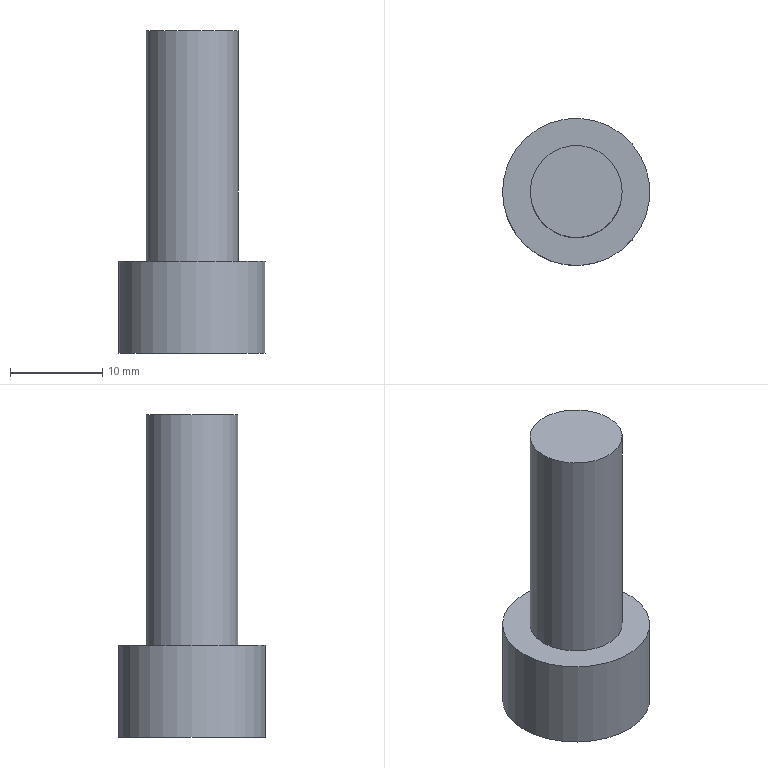Part | STEP file | 1 solid | 12 faces | box 16 x 16 x 35 mm | volume 3608 mm3 | plane 10 | cylinder 2 | commonest cylinder face diameters 10 x1 16 x1
STEP:
#1=CARTESIAN_POINT('',(0.,0.,0.));
#2=DIRECTION('',(0.,0.,1.));
#3=DIRECTION('',(1.,0.,0.));
#4=AXIS2_PLACEMENT_3D('',#1,#2,#3);
#5=CARTESIAN_POINT('',(1674.247,277.48,-164.381));
#6=VERTEX_POINT('',#5);
#7=CARTESIAN_POINT('',(1682.247,277.48,-164.381));
#8=DIRECTION('',(0.,0.,-1.));
#9=DIRECTION('',(-1.,0.,0.));
#10=AXIS2_PLACEMENT_3D('',#7,#8,#9);
#11=CIRCLE('',#10,8.);
#12=CARTESIAN_POINT('',(1674.247,277.48,-164.381));
#13=DIRECTION('',(0.,0.,1.));
#14=DIRECTION('',(1.,0.,0.));
#15=AXIS2_PLACEMENT_3D('',#12,#13,#14);
#16=PLANE('',#15);
#17=CARTESIAN_POINT('',(0.,0.));
#18=CARTESIAN_POINT('',(0.,13.856));
#19=CARTESIAN_POINT('',(12.,6.928));
#20=CARTESIAN_POINT('',(24.,0.));
#21=CARTESIAN_POINT('',(12.,-6.928));
#22=CARTESIAN_POINT('',(0.,-13.856));
#23=CARTESIAN_POINT('',(0.,0.));
#24=(BOUNDED_CURVE()B_SPLINE_CURVE(2,(#17,#18,#19,#20,#21,#22,#23),.UNSPECIFIED.,.T.,.F.)B_SPLINE_CURVE_WITH_KNOTS((1,2,2,2,2,1),(-2.094,0.,2.094,4.189,6.283,8.378),.UNSPECIFIED.)CURVE()GEOMETRIC_REPRESENTATION_ITEM()RATIONAL_B_SPLINE_CURVE((1.,0.5,1.,0.5,1.,0.5,1.))REPRESENTATION_ITEM(''));
#25=(GEOMETRIC_REPRESENTATION_CONTEXT(2)PARAMETRIC_REPRESENTATION_CONTEXT()REPRESENTATION_CONTEXT('',''));
#26=DEFINITIONAL_REPRESENTATION('',(#24),#25);
#27=PCURVE('',#16,#26);
#28=CARTESIAN_POINT('',(1682.247,277.48,-145.481));
#29=DIRECTION('',(0.,0.,-1.));
#30=DIRECTION('',(-1.,0.,0.));
#31=AXIS2_PLACEMENT_3D('',#28,#29,#30);
#32=CYLINDRICAL_SURFACE('',#31,8.);
#33=CARTESIAN_POINT('',(0.,18.9));
#34=DIRECTION('',(1.,0.));
#35=VECTOR('',#34,1.);
#36=LINE('',#33,#35);
#37=(GEOMETRIC_REPRESENTATION_CONTEXT(2)PARAMETRIC_REPRESENTATION_CONTEXT()REPRESENTATION_CONTEXT('',''));
#38=DEFINITIONAL_REPRESENTATION('',(#36),#37);
#39=PCURVE('',#32,#38);
#40=SURFACE_CURVE('',#11,(#27,#39),.PCURVE_S1.);
#41=EDGE_CURVE('',#6,#6,#40,.T.);
#42=ORIENTED_EDGE('',*,*,#41,.T.);
#43=EDGE_LOOP('',(#42));
#44=FACE_BOUND('',#43,.T.);
#45=CARTESIAN_POINT('',(1684.557,281.48,-164.381));
#46=VERTEX_POINT('',#45);
#47=CARTESIAN_POINT('',(1679.938,281.48,-164.381));
#48=VERTEX_POINT('',#47);
#49=CARTESIAN_POINT('',(1684.557,281.48,-164.381));
#50=DIRECTION('',(-1.,0.,0.));
#51=VECTOR('',#50,1.);
#52=LINE('',#49,#51);
#53=CARTESIAN_POINT('',(10.309,4.));
#54=DIRECTION('',(-1.,0.));
#55=VECTOR('',#54,1.);
#56=LINE('',#53,#55);
#57=(GEOMETRIC_REPRESENTATION_CONTEXT(2)PARAMETRIC_REPRESENTATION_CONTEXT()REPRESENTATION_CONTEXT('',''));
#58=DEFINITIONAL_REPRESENTATION('',(#56),#57);
#59=PCURVE('',#16,#58);
#60=CARTESIAN_POINT('',(1684.557,281.48,-157.781));
#61=DIRECTION('',(0.,-1.,0.));
#62=DIRECTION('',(-1.,0.,0.));
#63=AXIS2_PLACEMENT_3D('',#60,#61,#62);
#64=PLANE('',#63);
#65=CARTESIAN_POINT('',(0.,6.6));
#66=DIRECTION('',(1.,0.));
#67=VECTOR('',#66,1.);
#68=LINE('',#65,#67);
#69=(GEOMETRIC_REPRESENTATION_CONTEXT(2)PARAMETRIC_REPRESENTATION_CONTEXT()REPRESENTATION_CONTEXT('',''));
#70=DEFINITIONAL_REPRESENTATION('',(#68),#69);
#71=PCURVE('',#64,#70);
#72=SURFACE_CURVE('',#52,(#59,#71),.PCURVE_S1.);
#73=EDGE_CURVE('',#46,#48,#72,.T.);
#74=ORIENTED_EDGE('',*,*,#73,.T.);
#75=CARTESIAN_POINT('',(1677.628,277.48,-164.381));
#76=VERTEX_POINT('',#75);
#77=CARTESIAN_POINT('',(1679.938,281.48,-164.381));
#78=DIRECTION('',(-0.5,-0.866,0.));
#79=VECTOR('',#78,1.);
#80=LINE('',#77,#79);
#81=CARTESIAN_POINT('',(5.691,4.));
#82=DIRECTION('',(-0.5,-0.866));
#83=VECTOR('',#82,1.);
#84=LINE('',#81,#83);
#85=(GEOMETRIC_REPRESENTATION_CONTEXT(2)PARAMETRIC_REPRESENTATION_CONTEXT()REPRESENTATION_CONTEXT('',''));
#86=DEFINITIONAL_REPRESENTATION('',(#84),#85);
#87=PCURVE('',#16,#86);
#88=CARTESIAN_POINT('',(1679.938,281.48,-157.781));
#89=DIRECTION('',(0.866,-0.5,0.));
#90=DIRECTION('',(-0.5,-0.866,0.));
#91=AXIS2_PLACEMENT_3D('',#88,#89,#90);
#92=PLANE('',#91);
#93=CARTESIAN_POINT('',(0.,6.6));
#94=DIRECTION('',(1.,0.));
#95=VECTOR('',#94,1.);
#96=LINE('',#93,#95);
#97=(GEOMETRIC_REPRESENTATION_CONTEXT(2)PARAMETRIC_REPRESENTATION_CONTEXT()REPRESENTATION_CONTEXT('',''));
#98=DEFINITIONAL_REPRESENTATION('',(#96),#97);
#99=PCURVE('',#92,#98);
#100=SURFACE_CURVE('',#80,(#87,#99),.PCURVE_S1.);
#101=EDGE_CURVE('',#48,#76,#100,.T.);
#102=ORIENTED_EDGE('',*,*,#101,.T.);
#103=CARTESIAN_POINT('',(1679.938,273.48,-164.381));
#104=VERTEX_POINT('',#103);
#105=CARTESIAN_POINT('',(1677.628,277.48,-164.381));
#106=DIRECTION('',(0.5,-0.866,0.));
#107=VECTOR('',#106,1.);
#108=LINE('',#105,#107);
#109=CARTESIAN_POINT('',(3.381,0.));
#110=DIRECTION('',(0.5,-0.866));
#111=VECTOR('',#110,1.);
#112=LINE('',#109,#111);
#113=(GEOMETRIC_REPRESENTATION_CONTEXT(2)PARAMETRIC_REPRESENTATION_CONTEXT()REPRESENTATION_CONTEXT('',''));
#114=DEFINITIONAL_REPRESENTATION('',(#112),#113);
#115=PCURVE('',#16,#114);
#116=CARTESIAN_POINT('',(1677.628,277.48,-157.781));
#117=DIRECTION('',(0.866,0.5,0.));
#118=DIRECTION('',(0.5,-0.866,0.));
#119=AXIS2_PLACEMENT_3D('',#116,#117,#118);
#120=PLANE('',#119);
#121=CARTESIAN_POINT('',(0.,6.6));
#122=DIRECTION('',(1.,0.));
#123=VECTOR('',#122,1.);
#124=LINE('',#121,#123);
#125=(GEOMETRIC_REPRESENTATION_CONTEXT(2)PARAMETRIC_REPRESENTATION_CONTEXT()REPRESENTATION_CONTEXT('',''));
#126=DEFINITIONAL_REPRESENTATION('',(#124),#125);
#127=PCURVE('',#120,#126);
#128=SURFACE_CURVE('',#108,(#115,#127),.PCURVE_S1.);
#129=EDGE_CURVE('',#76,#104,#128,.T.);
#130=ORIENTED_EDGE('',*,*,#129,.T.);
#131=CARTESIAN_POINT('',(1684.557,273.48,-164.381));
#132=VERTEX_POINT('',#131);
#133=CARTESIAN_POINT('',(1679.938,273.48,-164.381));
#134=DIRECTION('',(1.,0.,0.));
#135=VECTOR('',#134,1.);
#136=LINE('',#133,#135);
#137=CARTESIAN_POINT('',(5.691,-4.));
#138=DIRECTION('',(1.,0.));
#139=VECTOR('',#138,1.);
#140=LINE('',#137,#139);
#141=(GEOMETRIC_REPRESENTATION_CONTEXT(2)PARAMETRIC_REPRESENTATION_CONTEXT()REPRESENTATION_CONTEXT('',''));
#142=DEFINITIONAL_REPRESENTATION('',(#140),#141);
#143=PCURVE('',#16,#142);
#144=CARTESIAN_POINT('',(1679.938,273.48,-157.781));
#145=DIRECTION('',(0.,1.,0.));
#146=DIRECTION('',(1.,0.,0.));
#147=AXIS2_PLACEMENT_3D('',#144,#145,#146);
#148=PLANE('',#147);
#149=CARTESIAN_POINT('',(0.,6.6));
#150=DIRECTION('',(1.,0.));
#151=VECTOR('',#150,1.);
#152=LINE('',#149,#151);
#153=(GEOMETRIC_REPRESENTATION_CONTEXT(2)PARAMETRIC_REPRESENTATION_CONTEXT()REPRESENTATION_CONTEXT('',''));
#154=DEFINITIONAL_REPRESENTATION('',(#152),#153);
#155=PCURVE('',#148,#154);
#156=SURFACE_CURVE('',#136,(#143,#155),.PCURVE_S1.);
#157=EDGE_CURVE('',#104,#132,#156,.T.);
#158=ORIENTED_EDGE('',*,*,#157,.T.);
#159=CARTESIAN_POINT('',(1686.866,277.48,-164.381));
#160=VERTEX_POINT('',#159);
#161=CARTESIAN_POINT('',(1684.557,273.48,-164.381));
#162=DIRECTION('',(0.5,0.866,0.));
#163=VECTOR('',#162,1.);
#164=LINE('',#161,#163);
#165=CARTESIAN_POINT('',(10.309,-4.));
#166=DIRECTION('',(0.5,0.866));
#167=VECTOR('',#166,1.);
#168=LINE('',#165,#167);
#169=(GEOMETRIC_REPRESENTATION_CONTEXT(2)PARAMETRIC_REPRESENTATION_CONTEXT()REPRESENTATION_CONTEXT('',''));
#170=DEFINITIONAL_REPRESENTATION('',(#168),#169);
#171=PCURVE('',#16,#170);
#172=CARTESIAN_POINT('',(1684.557,273.48,-157.781));
#173=DIRECTION('',(-0.866,0.5,0.));
#174=DIRECTION('',(0.5,0.866,0.));
#175=AXIS2_PLACEMENT_3D('',#172,#173,#174);
#176=PLANE('',#175);
#177=CARTESIAN_POINT('',(0.,6.6));
#178=DIRECTION('',(1.,0.));
#179=VECTOR('',#178,1.);
#180=LINE('',#177,#179);
#181=(GEOMETRIC_REPRESENTATION_CONTEXT(2)PARAMETRIC_REPRESENTATION_CONTEXT()REPRESENTATION_CONTEXT('',''));
#182=DEFINITIONAL_REPRESENTATION('',(#180),#181);
#183=PCURVE('',#176,#182);
#184=SURFACE_CURVE('',#164,(#171,#183),.PCURVE_S1.);
#185=EDGE_CURVE('',#132,#160,#184,.T.);
#186=ORIENTED_EDGE('',*,*,#185,.T.);
#187=CARTESIAN_POINT('',(1686.866,277.48,-164.381));
#188=DIRECTION('',(-0.5,0.866,0.));
#189=VECTOR('',#188,1.);
#190=LINE('',#187,#189);
#191=CARTESIAN_POINT('',(12.619,0.));
#192=DIRECTION('',(-0.5,0.866));
#193=VECTOR('',#192,1.);
#194=LINE('',#191,#193);
#195=(GEOMETRIC_REPRESENTATION_CONTEXT(2)PARAMETRIC_REPRESENTATION_CONTEXT()REPRESENTATION_CONTEXT('',''));
#196=DEFINITIONAL_REPRESENTATION('',(#194),#195);
#197=PCURVE('',#16,#196);
#198=CARTESIAN_POINT('',(1686.866,277.48,-157.781));
#199=DIRECTION('',(-0.866,-0.5,0.));
#200=DIRECTION('',(-0.5,0.866,0.));
#201=AXIS2_PLACEMENT_3D('',#198,#199,#200);
#202=PLANE('',#201);
#203=CARTESIAN_POINT('',(0.,6.6));
#204=DIRECTION('',(1.,0.));
#205=VECTOR('',#204,1.);
#206=LINE('',#203,#205);
#207=(GEOMETRIC_REPRESENTATION_CONTEXT(2)PARAMETRIC_REPRESENTATION_CONTEXT()REPRESENTATION_CONTEXT('',''));
#208=DEFINITIONAL_REPRESENTATION('',(#206),#207);
#209=PCURVE('',#202,#208);
#210=SURFACE_CURVE('',#190,(#197,#209),.PCURVE_S1.);
#211=EDGE_CURVE('',#160,#46,#210,.T.);
#212=ORIENTED_EDGE('',*,*,#211,.T.);
#213=EDGE_LOOP('',(#74,#102,#130,#158,#186,#212));
#214=FACE_BOUND('',#213,.T.);
#215=ADVANCED_FACE('',(#44,#214),#16,.F.);
#216=ORIENTED_EDGE('',*,*,#41,.F.);
#217=CARTESIAN_POINT('',(1674.247,277.48,-154.381));
#218=VERTEX_POINT('',#217);
#219=CARTESIAN_POINT('',(1674.247,277.48,-154.381));
#220=CARTESIAN_POINT('',(1674.247,277.48,-164.381));
#221=B_SPLINE_CURVE_WITH_KNOTS('',1,(#219,#220),.UNSPECIFIED.,.F.,.F.,(2,2),(8.9,18.9),.PIECEWISE_BEZIER_KNOTS.);
#222=CARTESIAN_POINT('',(0.,0.));
#223=DIRECTION('',(0.,1.));
#224=VECTOR('',#223,1.);
#225=LINE('',#222,#224);
#226=(GEOMETRIC_REPRESENTATION_CONTEXT(2)PARAMETRIC_REPRESENTATION_CONTEXT()REPRESENTATION_CONTEXT('',''));
#227=DEFINITIONAL_REPRESENTATION('',(#225),#226);
#228=PCURVE('',#32,#227);
#229=CARTESIAN_POINT('',(6.283,0.));
#230=DIRECTION('',(0.,1.));
#231=VECTOR('',#230,1.);
#232=LINE('',#229,#231);
#233=(GEOMETRIC_REPRESENTATION_CONTEXT(2)PARAMETRIC_REPRESENTATION_CONTEXT()REPRESENTATION_CONTEXT('',''));
#234=DEFINITIONAL_REPRESENTATION('',(#232),#233);
#235=PCURVE('',#32,#234);
#236=SEAM_CURVE('',#221,(#228,#235),.PCURVE_S1.);
#237=EDGE_CURVE('',#218,#6,#236,.T.);
#238=ORIENTED_EDGE('',*,*,#237,.F.);
#239=CARTESIAN_POINT('',(1682.247,277.48,-154.381));
#240=DIRECTION('',(0.,0.,-1.));
#241=DIRECTION('',(-1.,0.,0.));
#242=AXIS2_PLACEMENT_3D('',#239,#240,#241);
#243=CIRCLE('',#242,8.);
#244=CARTESIAN_POINT('',(0.,8.9));
#245=DIRECTION('',(1.,0.));
#246=VECTOR('',#245,1.);
#247=LINE('',#244,#246);
#248=(GEOMETRIC_REPRESENTATION_CONTEXT(2)PARAMETRIC_REPRESENTATION_CONTEXT()REPRESENTATION_CONTEXT('',''));
#249=DEFINITIONAL_REPRESENTATION('',(#247),#248);
#250=PCURVE('',#32,#249);
#251=CARTESIAN_POINT('',(1677.247,277.48,-154.381));
#252=DIRECTION('',(0.,0.,-1.));
#253=DIRECTION('',(-1.,0.,0.));
#254=AXIS2_PLACEMENT_3D('',#251,#252,#253);
#255=PLANE('',#254);
#256=CARTESIAN_POINT('',(-5.,0.));
#257=DIRECTION('',(1.,0.));
#258=AXIS2_PLACEMENT_2D('',#256,#257);
#259=CIRCLE('',#258,8.);
#260=(GEOMETRIC_REPRESENTATION_CONTEXT(2)PARAMETRIC_REPRESENTATION_CONTEXT()REPRESENTATION_CONTEXT('',''));
#261=DEFINITIONAL_REPRESENTATION('',(#259),#260);
#262=PCURVE('',#255,#261);
#263=SURFACE_CURVE('',#243,(#250,#262),.PCURVE_S1.);
#264=EDGE_CURVE('',#218,#218,#263,.T.);
#265=ORIENTED_EDGE('',*,*,#264,.T.);
#266=ORIENTED_EDGE('',*,*,#237,.T.);
#267=EDGE_LOOP('',(#216,#238,#265,#266));
#268=FACE_BOUND('',#267,.T.);
#269=ADVANCED_FACE('',(#268),#32,.T.);
#270=ORIENTED_EDGE('',*,*,#264,.F.);
#271=EDGE_LOOP('',(#270));
#272=FACE_BOUND('',#271,.T.);
#273=CARTESIAN_POINT('',(1677.247,277.48,-154.381));
#274=VERTEX_POINT('',#273);
#275=CARTESIAN_POINT('',(1682.247,277.48,-154.381));
#276=DIRECTION('',(0.,0.,-1.));
#277=DIRECTION('',(-1.,0.,0.));
#278=AXIS2_PLACEMENT_3D('',#275,#276,#277);
#279=CIRCLE('',#278,5.);
#280=CARTESIAN_POINT('',(-5.,0.));
#281=DIRECTION('',(1.,0.));
#282=AXIS2_PLACEMENT_2D('',#280,#281);
#283=CIRCLE('',#282,5.);
#284=(GEOMETRIC_REPRESENTATION_CONTEXT(2)PARAMETRIC_REPRESENTATION_CONTEXT()REPRESENTATION_CONTEXT('',''));
#285=DEFINITIONAL_REPRESENTATION('',(#283),#284);
#286=PCURVE('',#255,#285);
#287=CARTESIAN_POINT('',(1682.247,277.48,-145.481));
#288=DIRECTION('',(0.,0.,-1.));
#289=DIRECTION('',(-1.,0.,0.));
#290=AXIS2_PLACEMENT_3D('',#287,#288,#289);
#291=CYLINDRICAL_SURFACE('',#290,5.);
#292=CARTESIAN_POINT('',(0.,8.9));
#293=DIRECTION('',(1.,0.));
#294=VECTOR('',#293,1.);
#295=LINE('',#292,#294);
#296=(GEOMETRIC_REPRESENTATION_CONTEXT(2)PARAMETRIC_REPRESENTATION_CONTEXT()REPRESENTATION_CONTEXT('',''));
#297=DEFINITIONAL_REPRESENTATION('',(#295),#296);
#298=PCURVE('',#291,#297);
#299=SURFACE_CURVE('',#279,(#286,#298),.PCURVE_S1.);
#300=EDGE_CURVE('',#274,#274,#299,.T.);
#301=ORIENTED_EDGE('',*,*,#300,.T.);
#302=EDGE_LOOP('',(#301));
#303=FACE_BOUND('',#302,.T.);
#304=ADVANCED_FACE('',(#272,#303),#255,.F.);
#305=ORIENTED_EDGE('',*,*,#300,.F.);
#306=CARTESIAN_POINT('',(1677.247,277.48,-129.381));
#307=VERTEX_POINT('',#306);
#308=CARTESIAN_POINT('',(1677.247,277.48,-129.381));
#309=CARTESIAN_POINT('',(1677.247,277.48,-154.381));
#310=B_SPLINE_CURVE_WITH_KNOTS('',1,(#308,#309),.UNSPECIFIED.,.F.,.F.,(2,2),(-16.1,8.9),.PIECEWISE_BEZIER_KNOTS.);
#311=CARTESIAN_POINT('',(0.,0.));
#312=DIRECTION('',(0.,1.));
#313=VECTOR('',#312,1.);
#314=LINE('',#311,#313);
#315=(GEOMETRIC_REPRESENTATION_CONTEXT(2)PARAMETRIC_REPRESENTATION_CONTEXT()REPRESENTATION_CONTEXT('',''));
#316=DEFINITIONAL_REPRESENTATION('',(#314),#315);
#317=PCURVE('',#291,#316);
#318=CARTESIAN_POINT('',(6.283,0.));
#319=DIRECTION('',(0.,1.));
#320=VECTOR('',#319,1.);
#321=LINE('',#318,#320);
#322=(GEOMETRIC_REPRESENTATION_CONTEXT(2)PARAMETRIC_REPRESENTATION_CONTEXT()REPRESENTATION_CONTEXT('',''));
#323=DEFINITIONAL_REPRESENTATION('',(#321),#322);
#324=PCURVE('',#291,#323);
#325=SEAM_CURVE('',#310,(#317,#324),.PCURVE_S1.);
#326=EDGE_CURVE('',#307,#274,#325,.T.);
#327=ORIENTED_EDGE('',*,*,#326,.F.);
#328=CARTESIAN_POINT('',(1682.247,277.48,-129.381));
#329=DIRECTION('',(0.,0.,-1.));
#330=DIRECTION('',(-1.,0.,0.));
#331=AXIS2_PLACEMENT_3D('',#328,#329,#330);
#332=CIRCLE('',#331,5.);
#333=CARTESIAN_POINT('',(0.,-16.1));
#334=DIRECTION('',(1.,0.));
#335=VECTOR('',#334,1.);
#336=LINE('',#333,#335);
#337=(GEOMETRIC_REPRESENTATION_CONTEXT(2)PARAMETRIC_REPRESENTATION_CONTEXT()REPRESENTATION_CONTEXT('',''));
#338=DEFINITIONAL_REPRESENTATION('',(#336),#337);
#339=PCURVE('',#291,#338);
#340=CARTESIAN_POINT('',(1682.247,277.48,-129.381));
#341=DIRECTION('',(0.,0.,-1.));
#342=DIRECTION('',(-1.,0.,0.));
#343=AXIS2_PLACEMENT_3D('',#340,#341,#342);
#344=PLANE('',#343);
#345=CARTESIAN_POINT('',(0.,0.));
#346=DIRECTION('',(1.,0.));
#347=AXIS2_PLACEMENT_2D('',#345,#346);
#348=CIRCLE('',#347,5.);
#349=(GEOMETRIC_REPRESENTATION_CONTEXT(2)PARAMETRIC_REPRESENTATION_CONTEXT()REPRESENTATION_CONTEXT('',''));
#350=DEFINITIONAL_REPRESENTATION('',(#348),#349);
#351=PCURVE('',#344,#350);
#352=SURFACE_CURVE('',#332,(#339,#351),.PCURVE_S1.);
#353=EDGE_CURVE('',#307,#307,#352,.T.);
#354=ORIENTED_EDGE('',*,*,#353,.T.);
#355=ORIENTED_EDGE('',*,*,#326,.T.);
#356=EDGE_LOOP('',(#305,#327,#354,#355));
#357=FACE_BOUND('',#356,.T.);
#358=ADVANCED_FACE('',(#357),#291,.T.);
#359=ORIENTED_EDGE('',*,*,#353,.F.);
#360=EDGE_LOOP('',(#359));
#361=FACE_BOUND('',#360,.T.);
#362=ADVANCED_FACE('',(#361),#344,.F.);
#363=ORIENTED_EDGE('',*,*,#73,.F.);
#364=CARTESIAN_POINT('',(1684.557,281.48,-157.781));
#365=VERTEX_POINT('',#364);
#366=CARTESIAN_POINT('',(1684.557,281.48,-157.781));
#367=DIRECTION('',(0.,0.,1.));
#368=VECTOR('',#367,1.);
#369=LINE('',#366,#368);
#370=CARTESIAN_POINT('',(0.,0.));
#371=DIRECTION('',(0.,-1.));
#372=VECTOR('',#371,1.);
#373=LINE('',#370,#372);
#374=(GEOMETRIC_REPRESENTATION_CONTEXT(2)PARAMETRIC_REPRESENTATION_CONTEXT()REPRESENTATION_CONTEXT('',''));
#375=DEFINITIONAL_REPRESENTATION('',(#373),#374);
#376=PCURVE('',#64,#375);
#377=CARTESIAN_POINT('',(4.619,0.));
#378=DIRECTION('',(0.,-1.));
#379=VECTOR('',#378,1.);
#380=LINE('',#377,#379);
#381=(GEOMETRIC_REPRESENTATION_CONTEXT(2)PARAMETRIC_REPRESENTATION_CONTEXT()REPRESENTATION_CONTEXT('',''));
#382=DEFINITIONAL_REPRESENTATION('',(#380),#381);
#383=PCURVE('',#202,#382);
#384=SURFACE_CURVE('',#369,(#376,#383),.PCURVE_S1.);
#385=EDGE_CURVE('',#46,#365,#384,.T.);
#386=ORIENTED_EDGE('',*,*,#385,.T.);
#387=CARTESIAN_POINT('',(1679.938,281.48,-157.781));
#388=VERTEX_POINT('',#387);
#389=CARTESIAN_POINT('',(1684.557,281.48,-157.781));
#390=DIRECTION('',(1.,0.,0.));
#391=VECTOR('',#390,1.);
#392=LINE('',#389,#391);
#393=CARTESIAN_POINT('',(0.,0.));
#394=DIRECTION('',(-1.,0.));
#395=VECTOR('',#394,1.);
#396=LINE('',#393,#395);
#397=(GEOMETRIC_REPRESENTATION_CONTEXT(2)PARAMETRIC_REPRESENTATION_CONTEXT()REPRESENTATION_CONTEXT('',''));
#398=DEFINITIONAL_REPRESENTATION('',(#396),#397);
#399=PCURVE('',#64,#398);
#400=CARTESIAN_POINT('',(1682.247,277.48,-157.781));
#401=DIRECTION('',(0.,0.,1.));
#402=DIRECTION('',(1.,0.,0.));
#403=AXIS2_PLACEMENT_3D('',#400,#401,#402);
#404=PLANE('',#403);
#405=CARTESIAN_POINT('',(2.309,4.));
#406=DIRECTION('',(1.,0.));
#407=VECTOR('',#406,1.);
#408=LINE('',#405,#407);
#409=(GEOMETRIC_REPRESENTATION_CONTEXT(2)PARAMETRIC_REPRESENTATION_CONTEXT()REPRESENTATION_CONTEXT('',''));
#410=DEFINITIONAL_REPRESENTATION('',(#408),#409);
#411=PCURVE('',#404,#410);
#412=SURFACE_CURVE('',#392,(#399,#411),.PCURVE_S1.);
#413=EDGE_CURVE('',#388,#365,#412,.T.);
#414=ORIENTED_EDGE('',*,*,#413,.F.);
#415=CARTESIAN_POINT('',(1679.938,281.48,-157.781));
#416=DIRECTION('',(0.,0.,1.));
#417=VECTOR('',#416,1.);
#418=LINE('',#415,#417);
#419=CARTESIAN_POINT('',(4.619,0.));
#420=DIRECTION('',(0.,-1.));
#421=VECTOR('',#420,1.);
#422=LINE('',#419,#421);
#423=(GEOMETRIC_REPRESENTATION_CONTEXT(2)PARAMETRIC_REPRESENTATION_CONTEXT()REPRESENTATION_CONTEXT('',''));
#424=DEFINITIONAL_REPRESENTATION('',(#422),#423);
#425=PCURVE('',#64,#424);
#426=CARTESIAN_POINT('',(0.,0.));
#427=DIRECTION('',(0.,-1.));
#428=VECTOR('',#427,1.);
#429=LINE('',#426,#428);
#430=(GEOMETRIC_REPRESENTATION_CONTEXT(2)PARAMETRIC_REPRESENTATION_CONTEXT()REPRESENTATION_CONTEXT('',''));
#431=DEFINITIONAL_REPRESENTATION('',(#429),#430);
#432=PCURVE('',#92,#431);
#433=SURFACE_CURVE('',#418,(#425,#432),.PCURVE_S1.);
#434=EDGE_CURVE('',#48,#388,#433,.T.);
#435=ORIENTED_EDGE('',*,*,#434,.F.);
#436=EDGE_LOOP('',(#363,#386,#414,#435));
#437=FACE_BOUND('',#436,.T.);
#438=ADVANCED_FACE('',(#437),#64,.T.);
#439=ORIENTED_EDGE('',*,*,#101,.F.);
#440=ORIENTED_EDGE('',*,*,#434,.T.);
#441=CARTESIAN_POINT('',(1677.628,277.48,-157.781));
#442=VERTEX_POINT('',#441);
#443=CARTESIAN_POINT('',(1679.938,281.48,-157.781));
#444=DIRECTION('',(0.5,0.866,0.));
#445=VECTOR('',#444,1.);
#446=LINE('',#443,#445);
#447=CARTESIAN_POINT('',(0.,0.));
#448=DIRECTION('',(-1.,0.));
#449=VECTOR('',#448,1.);
#450=LINE('',#447,#449);
#451=(GEOMETRIC_REPRESENTATION_CONTEXT(2)PARAMETRIC_REPRESENTATION_CONTEXT()REPRESENTATION_CONTEXT('',''));
#452=DEFINITIONAL_REPRESENTATION('',(#450),#451);
#453=PCURVE('',#92,#452);
#454=CARTESIAN_POINT('',(-2.309,4.));
#455=DIRECTION('',(0.5,0.866));
#456=VECTOR('',#455,1.);
#457=LINE('',#454,#456);
#458=(GEOMETRIC_REPRESENTATION_CONTEXT(2)PARAMETRIC_REPRESENTATION_CONTEXT()REPRESENTATION_CONTEXT('',''));
#459=DEFINITIONAL_REPRESENTATION('',(#457),#458);
#460=PCURVE('',#404,#459);
#461=SURFACE_CURVE('',#446,(#453,#460),.PCURVE_S1.);
#462=EDGE_CURVE('',#442,#388,#461,.T.);
#463=ORIENTED_EDGE('',*,*,#462,.F.);
#464=CARTESIAN_POINT('',(1677.628,277.48,-157.781));
#465=DIRECTION('',(0.,0.,1.));
#466=VECTOR('',#465,1.);
#467=LINE('',#464,#466);
#468=CARTESIAN_POINT('',(4.619,0.));
#469=DIRECTION('',(0.,-1.));
#470=VECTOR('',#469,1.);
#471=LINE('',#468,#470);
#472=(GEOMETRIC_REPRESENTATION_CONTEXT(2)PARAMETRIC_REPRESENTATION_CONTEXT()REPRESENTATION_CONTEXT('',''));
#473=DEFINITIONAL_REPRESENTATION('',(#471),#472);
#474=PCURVE('',#92,#473);
#475=CARTESIAN_POINT('',(0.,0.));
#476=DIRECTION('',(0.,-1.));
#477=VECTOR('',#476,1.);
#478=LINE('',#475,#477);
#479=(GEOMETRIC_REPRESENTATION_CONTEXT(2)PARAMETRIC_REPRESENTATION_CONTEXT()REPRESENTATION_CONTEXT('',''));
#480=DEFINITIONAL_REPRESENTATION('',(#478),#479);
#481=PCURVE('',#120,#480);
#482=SURFACE_CURVE('',#467,(#474,#481),.PCURVE_S1.);
#483=EDGE_CURVE('',#76,#442,#482,.T.);
#484=ORIENTED_EDGE('',*,*,#483,.F.);
#485=EDGE_LOOP('',(#439,#440,#463,#484));
#486=FACE_BOUND('',#485,.T.);
#487=ADVANCED_FACE('',(#486),#92,.T.);
#488=ORIENTED_EDGE('',*,*,#129,.F.);
#489=ORIENTED_EDGE('',*,*,#483,.T.);
#490=CARTESIAN_POINT('',(1679.938,273.48,-157.781));
#491=VERTEX_POINT('',#490);
#492=CARTESIAN_POINT('',(1677.628,277.48,-157.781));
#493=DIRECTION('',(-0.5,0.866,0.));
#494=VECTOR('',#493,1.);
#495=LINE('',#492,#494);
#496=CARTESIAN_POINT('',(0.,0.));
#497=DIRECTION('',(-1.,0.));
#498=VECTOR('',#497,1.);
#499=LINE('',#496,#498);
#500=(GEOMETRIC_REPRESENTATION_CONTEXT(2)PARAMETRIC_REPRESENTATION_CONTEXT()REPRESENTATION_CONTEXT('',''));
#501=DEFINITIONAL_REPRESENTATION('',(#499),#500);
#502=PCURVE('',#120,#501);
#503=CARTESIAN_POINT('',(-4.619,0.));
#504=DIRECTION('',(-0.5,0.866));
#505=VECTOR('',#504,1.);
#506=LINE('',#503,#505);
#507=(GEOMETRIC_REPRESENTATION_CONTEXT(2)PARAMETRIC_REPRESENTATION_CONTEXT()REPRESENTATION_CONTEXT('',''));
#508=DEFINITIONAL_REPRESENTATION('',(#506),#507);
#509=PCURVE('',#404,#508);
#510=SURFACE_CURVE('',#495,(#502,#509),.PCURVE_S1.);
#511=EDGE_CURVE('',#491,#442,#510,.T.);
#512=ORIENTED_EDGE('',*,*,#511,.F.);
#513=CARTESIAN_POINT('',(1679.938,273.48,-157.781));
#514=DIRECTION('',(0.,0.,1.));
#515=VECTOR('',#514,1.);
#516=LINE('',#513,#515);
#517=CARTESIAN_POINT('',(4.619,0.));
#518=DIRECTION('',(0.,-1.));
#519=VECTOR('',#518,1.);
#520=LINE('',#517,#519);
#521=(GEOMETRIC_REPRESENTATION_CONTEXT(2)PARAMETRIC_REPRESENTATION_CONTEXT()REPRESENTATION_CONTEXT('',''));
#522=DEFINITIONAL_REPRESENTATION('',(#520),#521);
#523=PCURVE('',#120,#522);
#524=CARTESIAN_POINT('',(0.,0.));
#525=DIRECTION('',(0.,-1.));
#526=VECTOR('',#525,1.);
#527=LINE('',#524,#526);
#528=(GEOMETRIC_REPRESENTATION_CONTEXT(2)PARAMETRIC_REPRESENTATION_CONTEXT()REPRESENTATION_CONTEXT('',''));
#529=DEFINITIONAL_REPRESENTATION('',(#527),#528);
#530=PCURVE('',#148,#529);
#531=SURFACE_CURVE('',#516,(#523,#530),.PCURVE_S1.);
#532=EDGE_CURVE('',#104,#491,#531,.T.);
#533=ORIENTED_EDGE('',*,*,#532,.F.);
#534=EDGE_LOOP('',(#488,#489,#512,#533));
#535=FACE_BOUND('',#534,.T.);
#536=ADVANCED_FACE('',(#535),#120,.T.);
#537=ORIENTED_EDGE('',*,*,#157,.F.);
#538=ORIENTED_EDGE('',*,*,#532,.T.);
#539=CARTESIAN_POINT('',(1684.557,273.48,-157.781));
#540=VERTEX_POINT('',#539);
#541=CARTESIAN_POINT('',(1679.938,273.48,-157.781));
#542=DIRECTION('',(-1.,0.,0.));
#543=VECTOR('',#542,1.);
#544=LINE('',#541,#543);
#545=CARTESIAN_POINT('',(0.,0.));
#546=DIRECTION('',(-1.,0.));
#547=VECTOR('',#546,1.);
#548=LINE('',#545,#547);
#549=(GEOMETRIC_REPRESENTATION_CONTEXT(2)PARAMETRIC_REPRESENTATION_CONTEXT()REPRESENTATION_CONTEXT('',''));
#550=DEFINITIONAL_REPRESENTATION('',(#548),#549);
#551=PCURVE('',#148,#550);
#552=CARTESIAN_POINT('',(-2.309,-4.));
#553=DIRECTION('',(-1.,0.));
#554=VECTOR('',#553,1.);
#555=LINE('',#552,#554);
#556=(GEOMETRIC_REPRESENTATION_CONTEXT(2)PARAMETRIC_REPRESENTATION_CONTEXT()REPRESENTATION_CONTEXT('',''));
#557=DEFINITIONAL_REPRESENTATION('',(#555),#556);
#558=PCURVE('',#404,#557);
#559=SURFACE_CURVE('',#544,(#551,#558),.PCURVE_S1.);
#560=EDGE_CURVE('',#540,#491,#559,.T.);
#561=ORIENTED_EDGE('',*,*,#560,.F.);
#562=CARTESIAN_POINT('',(1684.557,273.48,-157.781));
#563=DIRECTION('',(0.,0.,1.));
#564=VECTOR('',#563,1.);
#565=LINE('',#562,#564);
#566=CARTESIAN_POINT('',(4.619,0.));
#567=DIRECTION('',(0.,-1.));
#568=VECTOR('',#567,1.);
#569=LINE('',#566,#568);
#570=(GEOMETRIC_REPRESENTATION_CONTEXT(2)PARAMETRIC_REPRESENTATION_CONTEXT()REPRESENTATION_CONTEXT('',''));
#571=DEFINITIONAL_REPRESENTATION('',(#569),#570);
#572=PCURVE('',#148,#571);
#573=CARTESIAN_POINT('',(0.,0.));
#574=DIRECTION('',(0.,-1.));
#575=VECTOR('',#574,1.);
#576=LINE('',#573,#575);
#577=(GEOMETRIC_REPRESENTATION_CONTEXT(2)PARAMETRIC_REPRESENTATION_CONTEXT()REPRESENTATION_CONTEXT('',''));
#578=DEFINITIONAL_REPRESENTATION('',(#576),#577);
#579=PCURVE('',#176,#578);
#580=SURFACE_CURVE('',#565,(#572,#579),.PCURVE_S1.);
#581=EDGE_CURVE('',#132,#540,#580,.T.);
#582=ORIENTED_EDGE('',*,*,#581,.F.);
#583=EDGE_LOOP('',(#537,#538,#561,#582));
#584=FACE_BOUND('',#583,.T.);
#585=ADVANCED_FACE('',(#584),#148,.T.);
#586=ORIENTED_EDGE('',*,*,#185,.F.);
#587=ORIENTED_EDGE('',*,*,#581,.T.);
#588=CARTESIAN_POINT('',(1686.866,277.48,-157.781));
#589=VERTEX_POINT('',#588);
#590=CARTESIAN_POINT('',(1684.557,273.48,-157.781));
#591=DIRECTION('',(-0.5,-0.866,0.));
#592=VECTOR('',#591,1.);
#593=LINE('',#590,#592);
#594=CARTESIAN_POINT('',(0.,0.));
#595=DIRECTION('',(-1.,0.));
#596=VECTOR('',#595,1.);
#597=LINE('',#594,#596);
#598=(GEOMETRIC_REPRESENTATION_CONTEXT(2)PARAMETRIC_REPRESENTATION_CONTEXT()REPRESENTATION_CONTEXT('',''));
#599=DEFINITIONAL_REPRESENTATION('',(#597),#598);
#600=PCURVE('',#176,#599);
#601=CARTESIAN_POINT('',(2.309,-4.));
#602=DIRECTION('',(-0.5,-0.866));
#603=VECTOR('',#602,1.);
#604=LINE('',#601,#603);
#605=(GEOMETRIC_REPRESENTATION_CONTEXT(2)PARAMETRIC_REPRESENTATION_CONTEXT()REPRESENTATION_CONTEXT('',''));
#606=DEFINITIONAL_REPRESENTATION('',(#604),#605);
#607=PCURVE('',#404,#606);
#608=SURFACE_CURVE('',#593,(#600,#607),.PCURVE_S1.);
#609=EDGE_CURVE('',#589,#540,#608,.T.);
#610=ORIENTED_EDGE('',*,*,#609,.F.);
#611=CARTESIAN_POINT('',(1686.866,277.48,-157.781));
#612=DIRECTION('',(0.,0.,1.));
#613=VECTOR('',#612,1.);
#614=LINE('',#611,#613);
#615=CARTESIAN_POINT('',(4.619,0.));
#616=DIRECTION('',(0.,-1.));
#617=VECTOR('',#616,1.);
#618=LINE('',#615,#617);
#619=(GEOMETRIC_REPRESENTATION_CONTEXT(2)PARAMETRIC_REPRESENTATION_CONTEXT()REPRESENTATION_CONTEXT('',''));
#620=DEFINITIONAL_REPRESENTATION('',(#618),#619);
#621=PCURVE('',#176,#620);
#622=CARTESIAN_POINT('',(0.,0.));
#623=DIRECTION('',(0.,-1.));
#624=VECTOR('',#623,1.);
#625=LINE('',#622,#624);
#626=(GEOMETRIC_REPRESENTATION_CONTEXT(2)PARAMETRIC_REPRESENTATION_CONTEXT()REPRESENTATION_CONTEXT('',''));
#627=DEFINITIONAL_REPRESENTATION('',(#625),#626);
#628=PCURVE('',#202,#627);
#629=SURFACE_CURVE('',#614,(#621,#628),.PCURVE_S1.);
#630=EDGE_CURVE('',#160,#589,#629,.T.);
#631=ORIENTED_EDGE('',*,*,#630,.F.);
#632=EDGE_LOOP('',(#586,#587,#610,#631));
#633=FACE_BOUND('',#632,.T.);
#634=ADVANCED_FACE('',(#633),#176,.T.);
#635=ORIENTED_EDGE('',*,*,#211,.F.);
#636=ORIENTED_EDGE('',*,*,#630,.T.);
#637=CARTESIAN_POINT('',(1686.866,277.48,-157.781));
#638=DIRECTION('',(0.5,-0.866,0.));
#639=VECTOR('',#638,1.);
#640=LINE('',#637,#639);
#641=CARTESIAN_POINT('',(0.,0.));
#642=DIRECTION('',(-1.,0.));
#643=VECTOR('',#642,1.);
#644=LINE('',#641,#643);
#645=(GEOMETRIC_REPRESENTATION_CONTEXT(2)PARAMETRIC_REPRESENTATION_CONTEXT()REPRESENTATION_CONTEXT('',''));
#646=DEFINITIONAL_REPRESENTATION('',(#644),#645);
#647=PCURVE('',#202,#646);
#648=CARTESIAN_POINT('',(4.619,0.));
#649=DIRECTION('',(0.5,-0.866));
#650=VECTOR('',#649,1.);
#651=LINE('',#648,#650);
#652=(GEOMETRIC_REPRESENTATION_CONTEXT(2)PARAMETRIC_REPRESENTATION_CONTEXT()REPRESENTATION_CONTEXT('',''));
#653=DEFINITIONAL_REPRESENTATION('',(#651),#652);
#654=PCURVE('',#404,#653);
#655=SURFACE_CURVE('',#640,(#647,#654),.PCURVE_S1.);
#656=EDGE_CURVE('',#365,#589,#655,.T.);
#657=ORIENTED_EDGE('',*,*,#656,.F.);
#658=ORIENTED_EDGE('',*,*,#385,.F.);
#659=EDGE_LOOP('',(#635,#636,#657,#658));
#660=FACE_BOUND('',#659,.T.);
#661=ADVANCED_FACE('',(#660),#202,.T.);
#662=ORIENTED_EDGE('',*,*,#413,.T.);
#663=ORIENTED_EDGE('',*,*,#656,.T.);
#664=ORIENTED_EDGE('',*,*,#609,.T.);
#665=ORIENTED_EDGE('',*,*,#560,.T.);
#666=ORIENTED_EDGE('',*,*,#511,.T.);
#667=ORIENTED_EDGE('',*,*,#462,.T.);
#668=EDGE_LOOP('',(#662,#663,#664,#665,#666,#667));
#669=FACE_BOUND('',#668,.T.);
#670=ADVANCED_FACE('',(#669),#404,.F.);
#671=CLOSED_SHELL('',(#215,#269,#304,#358,#362,#438,#487,#536,#585,#634,#661,#670));
#672=MANIFOLD_SOLID_BREP('',#671);
#673=(LENGTH_UNIT()NAMED_UNIT(*)SI_UNIT(.MILLI.,.METRE.));
#674=UNCERTAINTY_MEASURE_WITH_UNIT(LENGTH_MEASURE(0.000002),#673,'','');
#675=(NAMED_UNIT(*)PLANE_ANGLE_UNIT()SI_UNIT($,.RADIAN.));
#676=(NAMED_UNIT(*)SI_UNIT($,.STERADIAN.)SOLID_ANGLE_UNIT());
#677=(GEOMETRIC_REPRESENTATION_CONTEXT(3)GLOBAL_UNCERTAINTY_ASSIGNED_CONTEXT((#674))GLOBAL_UNIT_ASSIGNED_CONTEXT((#673,#675,#676))REPRESENTATION_CONTEXT('',''));
#678=ADVANCED_BREP_SHAPE_REPRESENTATION('',(#4,#672),#677);